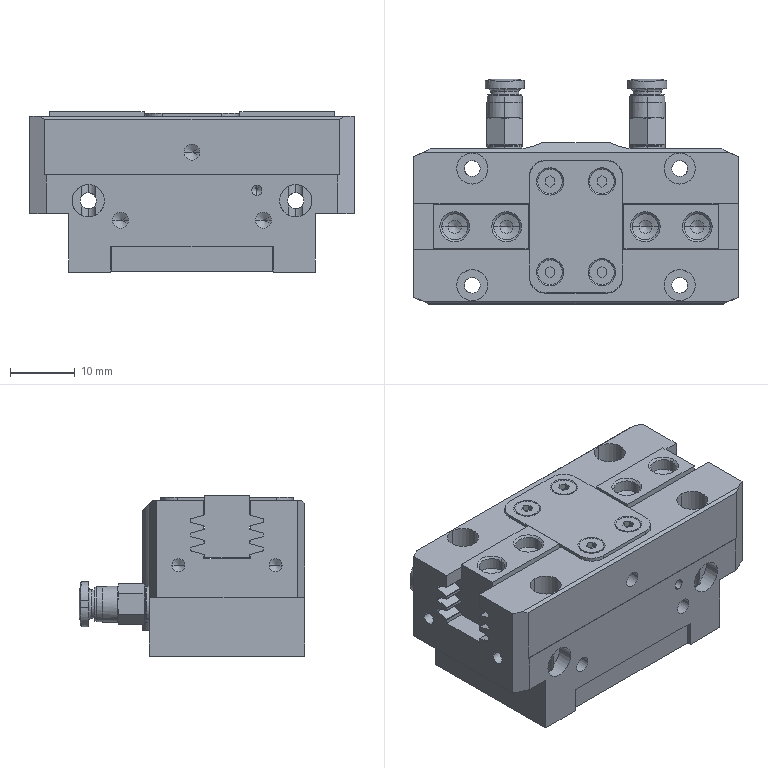Part | SolidWorks | 9 solids | 1612 faces | box 50 x 34.8 x 24.7 mm | volume 23663 mm3 | plane 1222 | cylinder 262 | cone 118 | spline 10 | commonest cylinder face diameters 0.2 x48 2.459 x26 0.4 x24 2.013 x18 1.567 x16 2.5 x12